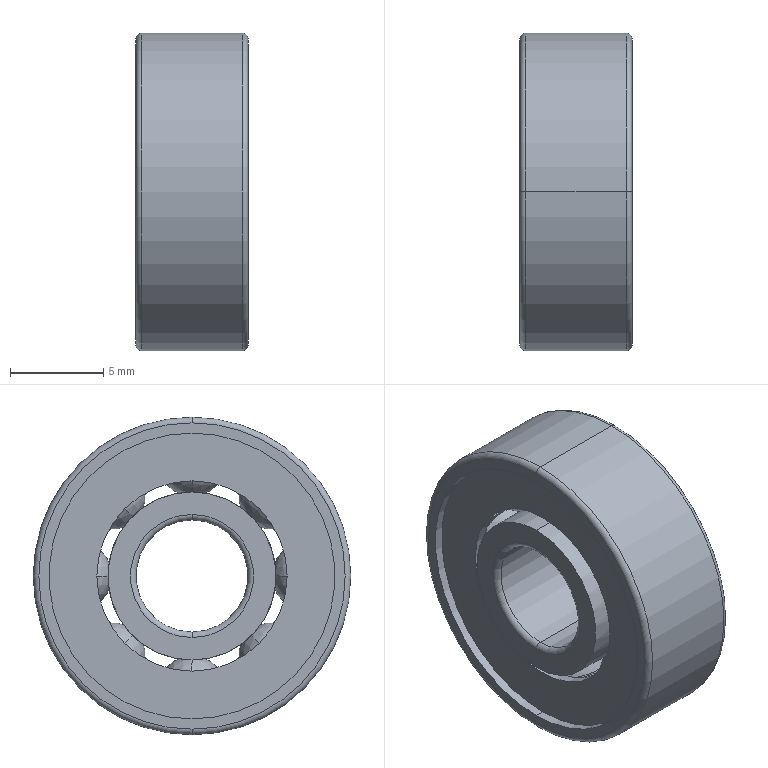Part | STEP file | Deep groove ball bearing 606-2Z | 1 solid | 144 faces | box 6 x 17 x 17 mm | volume 776.566 mm3 | sphere 64 | torus 32 | cylinder 24 | plane 24 | commonest cylinder face diameters 15.3 x8 9 x4 10.188 x4 6 x2 11.16 x2 13.14 x2